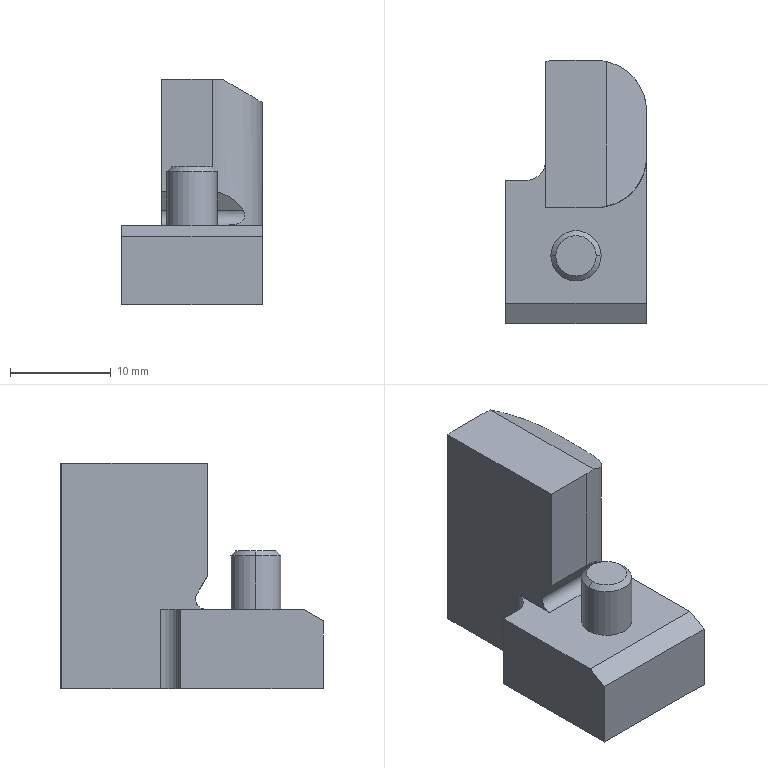Part | SolidWorks | features ICE 6, RefAxis 3, 3DProfileFeature 1, Extrusion 1, RevCut 1, Revolution 1 | 1 solid | 38 faces | box 14 x 26.1 x 22.4 mm | volume 4263 mm3 | plane 23 | cylinder 11 | cone 4 | commonest cylinder face diameters 10 x5 5 x2 8.5 x2 2 x1 4 x1
STEP:
#1=CARTESIAN_POINT('',(2.5,6.7,7.9));
#2=VERTEX_POINT('',#1);
#3=CARTESIAN_POINT('',(-2.5,6.7,7.9));
#4=VERTEX_POINT('',#3);
#5=CARTESIAN_POINT('',(0.,6.7,7.9));
#6=DIRECTION('',(0.,0.,1.));
#7=DIRECTION('',(-1.,0.,0.));
#8=AXIS2_PLACEMENT_3D('',#5,#6,#7);
#9=CIRCLE('',#8,2.5);
#10=EDGE_CURVE('',#2,#4,#9,.T.);
#11=ORIENTED_EDGE('',*,*,#10,.T.);
#12=CARTESIAN_POINT('',(-2.5,6.7,13.21));
#13=VERTEX_POINT('',#12);
#14=CARTESIAN_POINT('',(-2.5,6.7,7.9));
#15=DIRECTION('',(0.,0.,1.));
#16=VECTOR('',#15,1000.);
#17=LINE('',#14,#16);
#18=EDGE_CURVE('',#4,#13,#17,.T.);
#19=ORIENTED_EDGE('',*,*,#18,.T.);
#20=CARTESIAN_POINT('',(2.5,6.7,13.21));
#21=VERTEX_POINT('',#20);
#22=CARTESIAN_POINT('',(0.,6.7,13.21));
#23=DIRECTION('',(0.,0.,1.));
#24=DIRECTION('',(1.,0.,0.));
#25=AXIS2_PLACEMENT_3D('',#22,#23,#24);
#26=CIRCLE('',#25,2.5);
#27=EDGE_CURVE('',#21,#13,#26,.T.);
#28=ORIENTED_EDGE('',*,*,#27,.F.);
#29=CARTESIAN_POINT('',(2.5,6.7,7.9));
#30=DIRECTION('',(0.,0.,1.));
#31=VECTOR('',#30,1000.);
#32=LINE('',#29,#31);
#33=EDGE_CURVE('',#2,#21,#32,.T.);
#34=ORIENTED_EDGE('',*,*,#33,.F.);
#35=EDGE_LOOP('',(#11,#19,#28,#34));
#36=FACE_OUTER_BOUND('',#35,.T.);
#37=CARTESIAN_POINT('',(0.,6.7,7.9));
#38=DIRECTION('',(0.,0.,1.));
#39=DIRECTION('',(1.,0.,0.));
#40=AXIS2_PLACEMENT_3D('',#37,#38,#39);
#41=CYLINDRICAL_SURFACE('',#40,2.5);
#42=ADVANCED_FACE('',(#36),#41,.T.);
#43=CARTESIAN_POINT('',(2.01,6.7,13.7));
#44=VERTEX_POINT('',#43);
#45=CARTESIAN_POINT('',(-2.01,6.7,13.7));
#46=VERTEX_POINT('',#45);
#47=CARTESIAN_POINT('',(0.,6.7,13.7));
#48=DIRECTION('',(0.,0.,1.));
#49=DIRECTION('',(1.,0.,0.));
#50=AXIS2_PLACEMENT_3D('',#47,#48,#49);
#51=CIRCLE('',#50,2.01);
#52=EDGE_CURVE('',#44,#46,#51,.T.);
#53=ORIENTED_EDGE('',*,*,#52,.F.);
#54=CARTESIAN_POINT('',(2.5,6.7,13.21));
#55=DIRECTION('',(0.7071,0.,-0.7071));
#56=VECTOR('',#55,1000.);
#57=LINE('',#54,#56);
#58=EDGE_CURVE('',#44,#21,#57,.T.);
#59=ORIENTED_EDGE('',*,*,#58,.T.);
#60=ORIENTED_EDGE('',*,*,#27,.T.);
#61=CARTESIAN_POINT('',(-2.5,6.7,13.21));
#62=DIRECTION('',(-0.7071,0.,-0.7071));
#63=VECTOR('',#62,1000.);
#64=LINE('',#61,#63);
#65=EDGE_CURVE('',#46,#13,#64,.T.);
#66=ORIENTED_EDGE('',*,*,#65,.F.);
#67=EDGE_LOOP('',(#53,#59,#60,#66));
#68=FACE_OUTER_BOUND('',#67,.T.);
#69=CARTESIAN_POINT('',(0.,6.7,13.21));
#70=DIRECTION('',(0.,0.,-1.));
#71=DIRECTION('',(-1.,0.,0.));
#72=AXIS2_PLACEMENT_3D('',#69,#70,#71);
#73=CONICAL_SURFACE('',#72,2.5,0.7854);
#74=ADVANCED_FACE('',(#68),#73,.T.);
#75=CARTESIAN_POINT('',(-5.,6.7,0.));
#76=VERTEX_POINT('',#75);
#77=CARTESIAN_POINT('',(5.,6.7,0.));
#78=VERTEX_POINT('',#77);
#79=CARTESIAN_POINT('',(0.,6.7,0.));
#80=DIRECTION('',(0.,0.,1.));
#81=DIRECTION('',(1.,0.,0.));
#82=AXIS2_PLACEMENT_3D('',#79,#80,#81);
#83=CIRCLE('',#82,5.);
#84=EDGE_CURVE('',#76,#78,#83,.T.);
#85=ORIENTED_EDGE('',*,*,#84,.F.);
#86=CARTESIAN_POINT('',(-5.,6.7,5.7));
#87=VERTEX_POINT('',#86);
#88=CARTESIAN_POINT('',(-5.,6.7,0.));
#89=DIRECTION('',(0.,0.,1.));
#90=VECTOR('',#89,1000.);
#91=LINE('',#88,#90);
#92=EDGE_CURVE('',#76,#87,#91,.T.);
#93=ORIENTED_EDGE('',*,*,#92,.T.);
#94=CARTESIAN_POINT('',(5.,6.7,5.7));
#95=VERTEX_POINT('',#94);
#96=CARTESIAN_POINT('',(0.,6.7,5.7));
#97=DIRECTION('',(0.,0.,1.));
#98=DIRECTION('',(1.,0.,0.));
#99=AXIS2_PLACEMENT_3D('',#96,#97,#98);
#100=CIRCLE('',#99,5.);
#101=EDGE_CURVE('',#87,#95,#100,.T.);
#102=ORIENTED_EDGE('',*,*,#101,.T.);
#103=CARTESIAN_POINT('',(5.,6.7,0.));
#104=DIRECTION('',(0.,0.,1.));
#105=VECTOR('',#104,1000.);
#106=LINE('',#103,#105);
#107=EDGE_CURVE('',#78,#95,#106,.T.);
#108=ORIENTED_EDGE('',*,*,#107,.F.);
#109=EDGE_LOOP('',(#85,#93,#102,#108));
#110=FACE_OUTER_BOUND('',#109,.T.);
#111=CARTESIAN_POINT('',(0.,6.7,0.));
#112=DIRECTION('',(0.,0.,1.));
#113=DIRECTION('',(1.,0.,0.));
#114=AXIS2_PLACEMENT_3D('',#111,#112,#113);
#115=CYLINDRICAL_SURFACE('',#114,5.);
#116=ADVANCED_FACE('',(#110),#115,.F.);
#117=CARTESIAN_POINT('',(4.25,6.7,1.2));
#118=VERTEX_POINT('',#117);
#119=CARTESIAN_POINT('',(-4.25,6.7,1.2));
#120=VERTEX_POINT('',#119);
#121=CARTESIAN_POINT('',(0.,6.7,1.2));
#122=DIRECTION('',(0.,0.,1.));
#123=DIRECTION('',(1.,0.,0.));
#124=AXIS2_PLACEMENT_3D('',#121,#122,#123);
#125=CIRCLE('',#124,4.25);
#126=EDGE_CURVE('',#118,#120,#125,.T.);
#127=ORIENTED_EDGE('',*,*,#126,.T.);
#128=CARTESIAN_POINT('',(-4.25,6.7,5.7));
#129=VERTEX_POINT('',#128);
#130=CARTESIAN_POINT('',(-4.25,6.7,0.));
#131=DIRECTION('',(0.,0.,1.));
#132=VECTOR('',#131,1000.);
#133=LINE('',#130,#132);
#134=EDGE_CURVE('',#120,#129,#133,.T.);
#135=ORIENTED_EDGE('',*,*,#134,.T.);
#136=CARTESIAN_POINT('',(4.25,6.7,5.7));
#137=VERTEX_POINT('',#136);
#138=CARTESIAN_POINT('',(0.,6.7,5.7));
#139=DIRECTION('',(0.,0.,1.));
#140=DIRECTION('',(1.,0.,0.));
#141=AXIS2_PLACEMENT_3D('',#138,#139,#140);
#142=CIRCLE('',#141,4.25);
#143=EDGE_CURVE('',#137,#129,#142,.T.);
#144=ORIENTED_EDGE('',*,*,#143,.F.);
#145=CARTESIAN_POINT('',(4.25,6.7,0.));
#146=DIRECTION('',(0.,0.,1.));
#147=VECTOR('',#146,1000.);
#148=LINE('',#145,#147);
#149=EDGE_CURVE('',#118,#137,#148,.T.);
#150=ORIENTED_EDGE('',*,*,#149,.F.);
#151=EDGE_LOOP('',(#127,#135,#144,#150));
#152=FACE_OUTER_BOUND('',#151,.T.);
#153=CARTESIAN_POINT('',(0.,6.7,0.));
#154=DIRECTION('',(0.,0.,1.));
#155=DIRECTION('',(1.,0.,0.));
#156=AXIS2_PLACEMENT_3D('',#153,#154,#155);
#157=CYLINDRICAL_SURFACE('',#156,4.25);
#158=ADVANCED_FACE('',(#152),#157,.T.);
#159=CARTESIAN_POINT('',(3.75,6.7,0.7));
#160=VERTEX_POINT('',#159);
#161=CARTESIAN_POINT('',(-3.75,6.7,0.7));
#162=VERTEX_POINT('',#161);
#163=CARTESIAN_POINT('',(0.,6.7,0.7));
#164=DIRECTION('',(0.,0.,1.));
#165=DIRECTION('',(1.,0.,0.));
#166=AXIS2_PLACEMENT_3D('',#163,#164,#165);
#167=CIRCLE('',#166,3.75);
#168=EDGE_CURVE('',#160,#162,#167,.T.);
#169=ORIENTED_EDGE('',*,*,#168,.T.);
#170=CARTESIAN_POINT('',(-4.25,6.7,1.2));
#171=DIRECTION('',(-0.7071,0.,0.7071));
#172=VECTOR('',#171,1000.);
#173=LINE('',#170,#172);
#174=EDGE_CURVE('',#162,#120,#173,.T.);
#175=ORIENTED_EDGE('',*,*,#174,.T.);
#176=ORIENTED_EDGE('',*,*,#126,.F.);
#177=CARTESIAN_POINT('',(4.25,6.7,1.2));
#178=DIRECTION('',(0.7071,0.,0.7071));
#179=VECTOR('',#178,1000.);
#180=LINE('',#177,#179);
#181=EDGE_CURVE('',#160,#118,#180,.T.);
#182=ORIENTED_EDGE('',*,*,#181,.F.);
#183=EDGE_LOOP('',(#169,#175,#176,#182));
#184=FACE_OUTER_BOUND('',#183,.T.);
#185=CARTESIAN_POINT('',(0.,6.7,1.2));
#186=DIRECTION('',(0.,0.,1.));
#187=DIRECTION('',(1.,0.,0.));
#188=AXIS2_PLACEMENT_3D('',#185,#186,#187);
#189=CONICAL_SURFACE('',#188,4.25,0.7854);
#190=ADVANCED_FACE('',(#184),#189,.T.);
#191=CARTESIAN_POINT('',(-3.,11.7,7.9));
#192=VERTEX_POINT('',#191);
#193=CARTESIAN_POINT('',(3.4,11.7,7.9));
#194=VERTEX_POINT('',#193);
#195=CARTESIAN_POINT('',(-7.,11.7,7.9));
#196=DIRECTION('',(1.,0.,0.));
#197=VECTOR('',#196,1000.);
#198=LINE('',#195,#197);
#199=EDGE_CURVE('',#192,#194,#198,.T.);
#200=ORIENTED_EDGE('',*,*,#199,.F.);
#201=CARTESIAN_POINT('',(-3.,16.2,7.9));
#202=VERTEX_POINT('',#201);
#203=CARTESIAN_POINT('',(-3.,11.5,7.9));
#204=DIRECTION('',(0.,1.,0.));
#205=VECTOR('',#204,1000.);
#206=LINE('',#203,#205);
#207=EDGE_CURVE('',#192,#202,#206,.T.);
#208=ORIENTED_EDGE('',*,*,#207,.T.);
#209=CARTESIAN_POINT('',(-5.,14.2,7.9));
#210=VERTEX_POINT('',#209);
#211=CARTESIAN_POINT('',(-5.,16.2,7.9));
#212=DIRECTION('',(0.,0.,-1.));
#213=DIRECTION('',(-1.,0.,0.));
#214=AXIS2_PLACEMENT_3D('',#211,#212,#213);
#215=CIRCLE('',#214,2.);
#216=EDGE_CURVE('',#202,#210,#215,.T.);
#217=ORIENTED_EDGE('',*,*,#216,.T.);
#218=CARTESIAN_POINT('',(-7.,14.2,7.9));
#219=VERTEX_POINT('',#218);
#220=CARTESIAN_POINT('',(2.,14.2,7.9));
#221=DIRECTION('',(-1.,0.,0.));
#222=VECTOR('',#221,1000.);
#223=LINE('',#220,#222);
#224=EDGE_CURVE('',#210,#219,#223,.T.);
#225=ORIENTED_EDGE('',*,*,#224,.T.);
#226=CARTESIAN_POINT('',(-7.,2.,7.9));
#227=VERTEX_POINT('',#226);
#228=CARTESIAN_POINT('',(-7.,26.1,7.9));
#229=DIRECTION('',(0.,-1.,0.));
#230=VECTOR('',#229,1000.);
#231=LINE('',#228,#230);
#232=EDGE_CURVE('',#219,#227,#231,.T.);
#233=ORIENTED_EDGE('',*,*,#232,.T.);
#234=CARTESIAN_POINT('',(7.,2.,7.9));
#235=VERTEX_POINT('',#234);
#236=CARTESIAN_POINT('',(-7.,2.,7.9));
#237=DIRECTION('',(1.,0.,0.));
#238=VECTOR('',#237,1000.);
#239=LINE('',#236,#238);
#240=EDGE_CURVE('',#227,#235,#239,.T.);
#241=ORIENTED_EDGE('',*,*,#240,.T.);
#242=CARTESIAN_POINT('',(7.,16.5,7.9));
#243=VERTEX_POINT('',#242);
#244=CARTESIAN_POINT('',(7.,0.,7.9));
#245=DIRECTION('',(0.,-1.,0.));
#246=VECTOR('',#245,1000.);
#247=LINE('',#244,#246);
#248=EDGE_CURVE('',#243,#235,#247,.T.);
#249=ORIENTED_EDGE('',*,*,#248,.F.);
#250=CARTESIAN_POINT('',(2.,16.5,7.9));
#251=DIRECTION('',(0.,0.,-1.));
#252=DIRECTION('',(-1.,0.,0.));
#253=AXIS2_PLACEMENT_3D('',#250,#251,#252);
#254=CIRCLE('',#253,5.);
#255=EDGE_CURVE('',#243,#194,#254,.T.);
#256=ORIENTED_EDGE('',*,*,#255,.T.);
#257=EDGE_LOOP('',(#200,#208,#217,#225,#233,#241,#249,#256));
#258=FACE_OUTER_BOUND('',#257,.T.);
#259=ORIENTED_EDGE('',*,*,#10,.F.);
#260=CARTESIAN_POINT('',(0.,6.7,7.9));
#261=DIRECTION('',(0.,0.,1.));
#262=DIRECTION('',(-1.,0.,0.));
#263=AXIS2_PLACEMENT_3D('',#260,#261,#262);
#264=CIRCLE('',#263,2.5);
#265=EDGE_CURVE('',#4,#2,#264,.T.);
#266=ORIENTED_EDGE('',*,*,#265,.F.);
#267=EDGE_LOOP('',(#259,#266));
#268=FACE_BOUND('',#267,.T.);
#269=CARTESIAN_POINT('',(2.,16.5,7.9));
#270=DIRECTION('',(0.,0.,-1.));
#271=DIRECTION('',(-1.,0.,0.));
#272=AXIS2_PLACEMENT_3D('',#269,#270,#271);
#273=PLANE('',#272);
#274=ADVANCED_FACE('',(#258,#268),#273,.F.);
#275=CARTESIAN_POINT('',(-5.,14.2,0.));
#276=VERTEX_POINT('',#275);
#277=CARTESIAN_POINT('',(-3.,16.2,0.));
#278=VERTEX_POINT('',#277);
#279=CARTESIAN_POINT('',(-5.,16.2,0.));
#280=DIRECTION('',(0.,0.,1.));
#281=DIRECTION('',(1.,0.,0.));
#282=AXIS2_PLACEMENT_3D('',#279,#280,#281);
#283=CIRCLE('',#282,2.);
#284=EDGE_CURVE('',#276,#278,#283,.T.);
#285=ORIENTED_EDGE('',*,*,#284,.T.);
#286=CARTESIAN_POINT('',(-3.,25.999,0.));
#287=VERTEX_POINT('',#286);
#288=CARTESIAN_POINT('',(-3.,16.2,0.));
#289=DIRECTION('',(0.,1.,0.));
#290=VECTOR('',#289,1000.);
#291=LINE('',#288,#290);
#292=EDGE_CURVE('',#278,#287,#291,.T.);
#293=ORIENTED_EDGE('',*,*,#292,.T.);
#294=CARTESIAN_POINT('',(-2.,26.1,0.));
#295=VERTEX_POINT('',#294);
#296=CARTESIAN_POINT('',(-2.,21.1,0.));
#297=DIRECTION('',(0.,0.,1.));
#298=DIRECTION('',(1.,0.,0.));
#299=AXIS2_PLACEMENT_3D('',#296,#297,#298);
#300=CIRCLE('',#299,5.);
#301=EDGE_CURVE('',#295,#287,#300,.T.);
#302=ORIENTED_EDGE('',*,*,#301,.F.);
#303=CARTESIAN_POINT('',(2.,26.1,0.));
#304=VERTEX_POINT('',#303);
#305=CARTESIAN_POINT('',(2.,26.1,0.));
#306=DIRECTION('',(-1.,0.,0.));
#307=VECTOR('',#306,1000.);
#308=LINE('',#305,#307);
#309=EDGE_CURVE('',#304,#295,#308,.T.);
#310=ORIENTED_EDGE('',*,*,#309,.F.);
#311=CARTESIAN_POINT('',(7.,21.1,0.));
#312=VERTEX_POINT('',#311);
#313=CARTESIAN_POINT('',(2.,21.1,0.));
#314=DIRECTION('',(0.,0.,1.));
#315=DIRECTION('',(1.,0.,0.));
#316=AXIS2_PLACEMENT_3D('',#313,#314,#315);
#317=CIRCLE('',#316,5.);
#318=EDGE_CURVE('',#312,#304,#317,.T.);
#319=ORIENTED_EDGE('',*,*,#318,.F.);
#320=CARTESIAN_POINT('',(7.,0.,0.));
#321=VERTEX_POINT('',#320);
#322=CARTESIAN_POINT('',(7.,0.,0.));
#323=DIRECTION('',(0.,1.,0.));
#324=VECTOR('',#323,1000.);
#325=LINE('',#322,#324);
#326=EDGE_CURVE('',#321,#312,#325,.T.);
#327=ORIENTED_EDGE('',*,*,#326,.F.);
#328=CARTESIAN_POINT('',(-7.,0.,0.));
#329=VERTEX_POINT('',#328);
#330=CARTESIAN_POINT('',(-7.,0.,0.));
#331=DIRECTION('',(1.,0.,0.));
#332=VECTOR('',#331,1000.);
#333=LINE('',#330,#332);
#334=EDGE_CURVE('',#329,#321,#333,.T.);
#335=ORIENTED_EDGE('',*,*,#334,.F.);
#336=CARTESIAN_POINT('',(-7.,14.2,0.));
#337=VERTEX_POINT('',#336);
#338=CARTESIAN_POINT('',(-7.,21.1,0.));
#339=DIRECTION('',(0.,-1.,0.));
#340=VECTOR('',#339,1000.);
#341=LINE('',#338,#340);
#342=EDGE_CURVE('',#337,#329,#341,.T.);
#343=ORIENTED_EDGE('',*,*,#342,.F.);
#344=CARTESIAN_POINT('',(-7.,14.2,0.));
#345=DIRECTION('',(1.,0.,0.));
#346=VECTOR('',#345,1000.);
#347=LINE('',#344,#346);
#348=EDGE_CURVE('',#337,#276,#347,.T.);
#349=ORIENTED_EDGE('',*,*,#348,.T.);
#350=EDGE_LOOP('',(#285,#293,#302,#310,#319,#327,#335,#343,#349));
#351=FACE_OUTER_BOUND('',#350,.T.);
#352=CARTESIAN_POINT('',(0.,6.7,0.));
#353=DIRECTION('',(0.,0.,1.));
#354=DIRECTION('',(1.,0.,0.));
#355=AXIS2_PLACEMENT_3D('',#352,#353,#354);
#356=CIRCLE('',#355,5.);
#357=EDGE_CURVE('',#78,#76,#356,.T.);
#358=ORIENTED_EDGE('',*,*,#357,.T.);
#359=ORIENTED_EDGE('',*,*,#84,.T.);
#360=EDGE_LOOP('',(#358,#359));
#361=FACE_BOUND('',#360,.T.);
#362=CARTESIAN_POINT('',(-2.,21.1,0.));
#363=DIRECTION('',(0.,0.,1.));
#364=DIRECTION('',(1.,0.,0.));
#365=AXIS2_PLACEMENT_3D('',#362,#363,#364);
#366=PLANE('',#365);
#367=ADVANCED_FACE('',(#351,#361),#366,.F.);
#368=ORIENTED_EDGE('',*,*,#301,.T.);
#369=CARTESIAN_POINT('',(-3.,25.999,22.4));
#370=VERTEX_POINT('',#369);
#371=CARTESIAN_POINT('',(-3.,25.999,22.4));
#372=DIRECTION('',(0.,0.,-1.));
#373=VECTOR('',#372,1000.);
#374=LINE('',#371,#373);
#375=EDGE_CURVE('',#370,#287,#374,.T.);
#376=ORIENTED_EDGE('',*,*,#375,.F.);
#377=CARTESIAN_POINT('',(-2.,26.1,22.4));
#378=VERTEX_POINT('',#377);
#379=CARTESIAN_POINT('',(-2.,21.1,22.4));
#380=DIRECTION('',(0.,0.,1.));
#381=DIRECTION('',(1.,0.,0.));
#382=AXIS2_PLACEMENT_3D('',#379,#380,#381);
#383=CIRCLE('',#382,5.);
#384=EDGE_CURVE('',#378,#370,#383,.T.);
#385=ORIENTED_EDGE('',*,*,#384,.F.);
#386=CARTESIAN_POINT('',(-2.,26.1,22.4));
#387=DIRECTION('',(0.,0.,-1.));
#388=VECTOR('',#387,1000.);
#389=LINE('',#386,#388);
#390=EDGE_CURVE('',#378,#295,#389,.T.);
#391=ORIENTED_EDGE('',*,*,#390,.T.);
#392=EDGE_LOOP('',(#368,#376,#385,#391));
#393=FACE_OUTER_BOUND('',#392,.T.);
#394=CARTESIAN_POINT('',(-2.,21.1,22.4));
#395=DIRECTION('',(0.,0.,-1.));
#396=DIRECTION('',(-1.,0.,0.));
#397=AXIS2_PLACEMENT_3D('',#394,#395,#396);
#398=CYLINDRICAL_SURFACE('',#397,5.);
#399=ADVANCED_FACE('',(#393),#398,.T.);
#400=CARTESIAN_POINT('',(3.016,11.604,22.4));
#401=VERTEX_POINT('',#400);
#402=CARTESIAN_POINT('',(3.016,25.996,22.4));
#403=VERTEX_POINT('',#402);
#404=CARTESIAN_POINT('',(3.016,-26.1,22.4));
#405=DIRECTION('',(0.,1.,0.));
#406=VECTOR('',#405,1000.);
#407=LINE('',#404,#406);
#408=EDGE_CURVE('',#401,#403,#407,.T.);
#409=ORIENTED_EDGE('',*,*,#408,.T.);
#410=CARTESIAN_POINT('',(2.,26.1,22.4));
#411=VERTEX_POINT('',#410);
#412=CARTESIAN_POINT('',(2.,21.1,22.4));
#413=DIRECTION('',(0.,0.,1.));
#414=DIRECTION('',(1.,0.,0.));
#415=AXIS2_PLACEMENT_3D('',#412,#413,#414);
#416=CIRCLE('',#415,5.);
#417=EDGE_CURVE('',#403,#411,#416,.T.);
#418=ORIENTED_EDGE('',*,*,#417,.T.);
#419=CARTESIAN_POINT('',(2.,26.1,22.4));
#420=DIRECTION('',(-1.,0.,0.));
#421=VECTOR('',#420,1000.);
#422=LINE('',#419,#421);
#423=EDGE_CURVE('',#411,#378,#422,.T.);
#424=ORIENTED_EDGE('',*,*,#423,.T.);
#425=ORIENTED_EDGE('',*,*,#384,.T.);
#426=CARTESIAN_POINT('',(-3.,11.5,22.4));
#427=VERTEX_POINT('',#426);
#428=CARTESIAN_POINT('',(-3.,21.1,22.4));
#429=DIRECTION('',(0.,-1.,0.));
#430=VECTOR('',#429,1000.);
#431=LINE('',#428,#430);
#432=EDGE_CURVE('',#370,#427,#431,.T.);
#433=ORIENTED_EDGE('',*,*,#432,.T.);
#434=CARTESIAN_POINT('',(2.,11.5,22.4));
#435=VERTEX_POINT('',#434);
#436=CARTESIAN_POINT('',(-2.,11.5,22.4));
#437=DIRECTION('',(1.,0.,0.));
#438=VECTOR('',#437,1000.);
#439=LINE('',#436,#438);
#440=EDGE_CURVE('',#427,#435,#439,.T.);
#441=ORIENTED_EDGE('',*,*,#440,.T.);
#442=CARTESIAN_POINT('',(2.,16.5,22.4));
#443=DIRECTION('',(0.,0.,1.));
#444=DIRECTION('',(1.,0.,0.));
#445=AXIS2_PLACEMENT_3D('',#442,#443,#444);
#446=CIRCLE('',#445,5.);
#447=EDGE_CURVE('',#435,#401,#446,.T.);
#448=ORIENTED_EDGE('',*,*,#447,.T.);
#449=EDGE_LOOP('',(#409,#418,#424,#425,#433,#441,#448));
#450=FACE_OUTER_BOUND('',#449,.T.);
#451=CARTESIAN_POINT('',(-2.,21.1,22.4));
#452=DIRECTION('',(0.,0.,1.));
#453=DIRECTION('',(1.,0.,0.));
#454=AXIS2_PLACEMENT_3D('',#451,#452,#453);
#455=PLANE('',#454);
#456=ADVANCED_FACE('',(#450),#455,.T.);
#457=CARTESIAN_POINT('',(7.,0.,6.745));
#458=VERTEX_POINT('',#457);
#459=CARTESIAN_POINT('',(7.,0.,22.4));
#460=DIRECTION('',(0.,0.,-1.));
#461=VECTOR('',#460,1000.);
#462=LINE('',#459,#461);
#463=EDGE_CURVE('',#458,#321,#462,.T.);
#464=ORIENTED_EDGE('',*,*,#463,.F.);
#465=CARTESIAN_POINT('',(-7.,0.,6.745));
#466=VERTEX_POINT('',#465);
#467=CARTESIAN_POINT('',(-7.,0.,6.745));
#468=DIRECTION('',(1.,0.,0.));
#469=VECTOR('',#468,1000.);
#470=LINE('',#467,#469);
#471=EDGE_CURVE('',#466,#458,#470,.T.);
#472=ORIENTED_EDGE('',*,*,#471,.F.);
#473=CARTESIAN_POINT('',(-7.,0.,22.4));
#474=DIRECTION('',(0.,0.,-1.));
#475=VECTOR('',#474,1000.);
#476=LINE('',#473,#475);
#477=EDGE_CURVE('',#466,#329,#476,.T.);
#478=ORIENTED_EDGE('',*,*,#477,.T.);
#479=ORIENTED_EDGE('',*,*,#334,.T.);
#480=EDGE_LOOP('',(#464,#472,#478,#479));
#481=FACE_OUTER_BOUND('',#480,.T.);
#482=CARTESIAN_POINT('',(-7.,0.,22.4));
#483=DIRECTION('',(0.,1.,0.));
#484=DIRECTION('',(0.,0.,1.));
#485=AXIS2_PLACEMENT_3D('',#482,#483,#484);
#486=PLANE('',#485);
#487=ADVANCED_FACE('',(#481),#486,.F.);
#488=ORIENTED_EDGE('',*,*,#232,.F.);
#489=CARTESIAN_POINT('',(-7.,14.2,0.));
#490=DIRECTION('',(0.,0.,1.));
#491=VECTOR('',#490,1000.);
#492=LINE('',#489,#491);
#493=EDGE_CURVE('',#337,#219,#492,.T.);
#494=ORIENTED_EDGE('',*,*,#493,.F.);
#495=ORIENTED_EDGE('',*,*,#342,.T.);
#496=ORIENTED_EDGE('',*,*,#477,.F.);
#497=CARTESIAN_POINT('',(-7.,0.,6.745));
#498=DIRECTION('',(0.,0.866,0.5));
#499=VECTOR('',#498,1000.);
#500=LINE('',#497,#499);
#501=EDGE_CURVE('',#466,#227,#500,.T.);
#502=ORIENTED_EDGE('',*,*,#501,.T.);
#503=EDGE_LOOP('',(#488,#494,#495,#496,#502));
#504=FACE_OUTER_BOUND('',#503,.T.);
#505=CARTESIAN_POINT('',(-7.,21.1,22.4));
#506=DIRECTION('',(1.,0.,0.));
#507=DIRECTION('',(0.,0.,-1.));
#508=AXIS2_PLACEMENT_3D('',#505,#506,#507);
#509=PLANE('',#508);
#510=ADVANCED_FACE('',(#504),#509,.F.);
#511=CARTESIAN_POINT('',(7.,21.1,20.1));
#512=VERTEX_POINT('',#511);
#513=CARTESIAN_POINT('',(7.,21.1,22.4));
#514=DIRECTION('',(0.,0.,-1.));
#515=VECTOR('',#514,1000.);
#516=LINE('',#513,#515);
#517=EDGE_CURVE('',#512,#312,#516,.T.);
#518=ORIENTED_EDGE('',*,*,#517,.F.);
#519=CARTESIAN_POINT('',(7.,16.5,20.1));
#520=VERTEX_POINT('',#519);
#521=CARTESIAN_POINT('',(7.,-26.1,20.1));
#522=DIRECTION('',(0.,1.,0.));
#523=VECTOR('',#522,1000.);
#524=LINE('',#521,#523);
#525=EDGE_CURVE('',#520,#512,#524,.T.);
#526=ORIENTED_EDGE('',*,*,#525,.F.);
#527=CARTESIAN_POINT('',(7.,16.5,27.7));
#528=DIRECTION('',(0.,0.,-1.));
#529=VECTOR('',#528,1000.);
#530=LINE('',#527,#529);
#531=EDGE_CURVE('',#520,#243,#530,.T.);
#532=ORIENTED_EDGE('',*,*,#531,.T.);
#533=ORIENTED_EDGE('',*,*,#248,.T.);
#534=CARTESIAN_POINT('',(7.,0.,6.745));
#535=DIRECTION('',(0.,0.866,0.5));
#536=VECTOR('',#535,1000.);
#537=LINE('',#534,#536);
#538=EDGE_CURVE('',#458,#235,#537,.T.);
#539=ORIENTED_EDGE('',*,*,#538,.F.);
#540=ORIENTED_EDGE('',*,*,#463,.T.);
#541=ORIENTED_EDGE('',*,*,#326,.T.);
#542=EDGE_LOOP('',(#518,#526,#532,#533,#539,#540,#541));
#543=FACE_OUTER_BOUND('',#542,.T.);
#544=CARTESIAN_POINT('',(7.,0.,22.4));
#545=DIRECTION('',(-1.,0.,0.));
#546=DIRECTION('',(0.,0.,1.));
#547=AXIS2_PLACEMENT_3D('',#544,#545,#546);
#548=PLANE('',#547);
#549=ADVANCED_FACE('',(#543),#548,.F.);
#550=ORIENTED_EDGE('',*,*,#417,.F.);
#551=CARTESIAN_POINT('',(3.016,25.996,22.4));
#552=CARTESIAN_POINT('',(5.439,25.493,21.002));
#553=CARTESIAN_POINT('',(7.,23.574,20.1));
#554=CARTESIAN_POINT('',(7.,21.1,20.1));
#555=(BOUNDED_CURVE()B_SPLINE_CURVE(3,(#551,#552,#553,#554),.UNSPECIFIED.,.F.,.F.)B_SPLINE_CURVE_WITH_KNOTS((4,4),(4.917,6.283),.UNSPECIFIED.)CURVE()GEOMETRIC_REPRESENTATION_ITEM()RATIONAL_B_SPLINE_CURVE((1.,0.8504,0.8504,1.))REPRESENTATION_ITEM(''));
#556=EDGE_CURVE('',#403,#512,#555,.T.);
#557=ORIENTED_EDGE('',*,*,#556,.T.);
#558=ORIENTED_EDGE('',*,*,#517,.T.);
#559=ORIENTED_EDGE('',*,*,#318,.T.);
#560=CARTESIAN_POINT('',(2.,26.1,22.4));
#561=DIRECTION('',(0.,0.,-1.));
#562=VECTOR('',#561,1000.);
#563=LINE('',#560,#562);
#564=EDGE_CURVE('',#411,#304,#563,.T.);
#565=ORIENTED_EDGE('',*,*,#564,.F.);
#566=EDGE_LOOP('',(#550,#557,#558,#559,#565));
#567=FACE_OUTER_BOUND('',#566,.T.);
#568=CARTESIAN_POINT('',(2.,21.1,22.4));
#569=DIRECTION('',(0.,0.,-1.));
#570=DIRECTION('',(-1.,0.,0.));
#571=AXIS2_PLACEMENT_3D('',#568,#569,#570);
#572=CYLINDRICAL_SURFACE('',#571,5.);
#573=ADVANCED_FACE('',(#567),#572,.T.);
#574=ORIENTED_EDGE('',*,*,#309,.T.);
#575=ORIENTED_EDGE('',*,*,#390,.F.);
#576=ORIENTED_EDGE('',*,*,#423,.F.);
#577=ORIENTED_EDGE('',*,*,#564,.T.);
#578=EDGE_LOOP('',(#574,#575,#576,#577));
#579=FACE_OUTER_BOUND('',#578,.T.);
#580=CARTESIAN_POINT('',(2.,26.1,22.4));
#581=DIRECTION('',(0.,-1.,0.));
#582=DIRECTION('',(0.,0.,-1.));
#583=AXIS2_PLACEMENT_3D('',#580,#581,#582);
#584=PLANE('',#583);
#585=ADVANCED_FACE('',(#579),#584,.F.);
#586=ORIENTED_EDGE('',*,*,#240,.F.);
#587=ORIENTED_EDGE('',*,*,#501,.F.);
#588=ORIENTED_EDGE('',*,*,#471,.T.);
#589=ORIENTED_EDGE('',*,*,#538,.T.);
#590=EDGE_LOOP('',(#586,#587,#588,#589));
#591=FACE_OUTER_BOUND('',#590,.T.);
#592=CARTESIAN_POINT('',(-7.,0.,6.745));
#593=DIRECTION('',(0.,0.5,-0.866));
#594=DIRECTION('',(0.,0.866,0.5));
#595=AXIS2_PLACEMENT_3D('',#592,#593,#594);
#596=PLANE('',#595);
#597=ADVANCED_FACE('',(#591),#596,.F.);
#598=CARTESIAN_POINT('',(-3.,11.5,11.246));
#599=VERTEX_POINT('',#598);
#600=CARTESIAN_POINT('',(-3.,12.566,9.4));
#601=VERTEX_POINT('',#600);
#602=CARTESIAN_POINT('',(-3.,4.375,23.587));
#603=DIRECTION('',(0.,0.5,-0.866));
#604=VECTOR('',#603,1000.);
#605=LINE('',#602,#604);
#606=EDGE_CURVE('',#599,#601,#605,.T.);
#607=ORIENTED_EDGE('',*,*,#606,.F.);
#608=CARTESIAN_POINT('',(-3.,11.5,27.7));
#609=DIRECTION('',(0.,0.,-1.));
#610=VECTOR('',#609,1000.);
#611=LINE('',#608,#610);
#612=EDGE_CURVE('',#427,#599,#611,.T.);
#613=ORIENTED_EDGE('',*,*,#612,.F.);
#614=ORIENTED_EDGE('',*,*,#432,.F.);
#615=ORIENTED_EDGE('',*,*,#375,.T.);
#616=ORIENTED_EDGE('',*,*,#292,.F.);
#617=CARTESIAN_POINT('',(-3.,16.2,0.));
#618=DIRECTION('',(0.,0.,1.));
#619=VECTOR('',#618,1000.);
#620=LINE('',#617,#619);
#621=EDGE_CURVE('',#278,#202,#620,.T.);
#622=ORIENTED_EDGE('',*,*,#621,.T.);
#623=ORIENTED_EDGE('',*,*,#207,.F.);
#624=CARTESIAN_POINT('',(-3.,11.7,8.9));
#625=DIRECTION('',(-1.,0.,0.));
#626=DIRECTION('',(0.,-1.,0.));
#627=AXIS2_PLACEMENT_3D('',#624,#625,#626);
#628=CIRCLE('',#627,1.);
#629=EDGE_CURVE('',#601,#192,#628,.T.);
#630=ORIENTED_EDGE('',*,*,#629,.F.);
#631=EDGE_LOOP('',(#607,#613,#614,#615,#616,#622,#623,#630));
#632=FACE_OUTER_BOUND('',#631,.T.);
#633=CARTESIAN_POINT('',(-3.,11.5,27.7));
#634=DIRECTION('',(-1.,0.,0.));
#635=DIRECTION('',(0.,-1.,0.));
#636=AXIS2_PLACEMENT_3D('',#633,#634,#635);
#637=PLANE('',#636);
#638=ADVANCED_FACE('',(#632),#637,.T.);
#639=CARTESIAN_POINT('',(3.016,11.604,22.4));
#640=CARTESIAN_POINT('',(5.439,12.107,21.002));
#641=CARTESIAN_POINT('',(7.,14.026,20.1));
#642=CARTESIAN_POINT('',(7.,16.5,20.1));
#643=(BOUNDED_CURVE()B_SPLINE_CURVE(3,(#639,#640,#641,#642),.UNSPECIFIED.,.F.,.T.)B_SPLINE_CURVE_WITH_KNOTS((4,4),(4.917,6.283),.UNSPECIFIED.)CURVE()GEOMETRIC_REPRESENTATION_ITEM()RATIONAL_B_SPLINE_CURVE((1.,0.8504,0.8504,1.))REPRESENTATION_ITEM(''));
#644=EDGE_CURVE('',#401,#520,#643,.T.);
#645=ORIENTED_EDGE('',*,*,#644,.F.);
#646=ORIENTED_EDGE('',*,*,#447,.F.);
#647=CARTESIAN_POINT('',(2.,11.5,11.246));
#648=VERTEX_POINT('',#647);
#649=CARTESIAN_POINT('',(2.,11.5,27.7));
#650=DIRECTION('',(0.,0.,-1.));
#651=VECTOR('',#650,1000.);
#652=LINE('',#649,#651);
#653=EDGE_CURVE('',#435,#648,#652,.T.);
#654=ORIENTED_EDGE('',*,*,#653,.T.);
#655=CARTESIAN_POINT('',(5.086,12.566,9.4));
#656=VERTEX_POINT('',#655);
#657=CARTESIAN_POINT('',(5.086,12.566,9.4));
#658=CARTESIAN_POINT('',(4.197,11.869,10.608));
#659=CARTESIAN_POINT('',(3.13,11.5,11.246));
#660=CARTESIAN_POINT('',(2.,11.5,11.246));
#661=(BOUNDED_CURVE()B_SPLINE_CURVE(3,(#657,#658,#659,#660),.UNSPECIFIED.,.F.,.F.)B_SPLINE_CURVE_WITH_KNOTS((4,4),(2.476,3.142),.UNSPECIFIED.)CURVE()GEOMETRIC_REPRESENTATION_ITEM()RATIONAL_B_SPLINE_CURVE((1.,0.9635,0.9635,1.))REPRESENTATION_ITEM(''));
#662=EDGE_CURVE('',#656,#648,#661,.T.);
#663=ORIENTED_EDGE('',*,*,#662,.F.);
#664=CARTESIAN_POINT('',(3.4,11.7,7.9));
#665=CARTESIAN_POINT('',(3.651,11.773,7.9));
#666=CARTESIAN_POINT('',(3.894,11.865,7.907));
#667=CARTESIAN_POINT('',(4.361,12.085,7.97));
#668=CARTESIAN_POINT('',(4.588,12.215,8.026));
#669=CARTESIAN_POINT('',(4.882,12.412,8.193));
#670=CARTESIAN_POINT('',(4.972,12.478,8.263));
#671=CARTESIAN_POINT('',(5.124,12.595,8.442));
#672=CARTESIAN_POINT('',(5.185,12.645,8.551));
#673=CARTESIAN_POINT('',(5.253,12.703,8.797));
#674=CARTESIAN_POINT('',(5.259,12.708,8.934));
#675=CARTESIAN_POINT('',(5.21,12.666,9.188));
#676=CARTESIAN_POINT('',(5.157,12.622,9.304));
#677=CARTESIAN_POINT('',(5.086,12.566,9.4));
#678=B_SPLINE_CURVE_WITH_KNOTS('',3,(#664,#665,#666,#667,#668,#669,#670,#671,#672,#673,#674,#675,#676,#677),.UNSPECIFIED.,.F.,.F.,(4,2,2,2,2,2,4),(0.,0.000778,0.001556,0.001945,0.002334,0.002723,0.003112),.UNSPECIFIED.);
#679=EDGE_CURVE('',#194,#656,#678,.T.);
#680=ORIENTED_EDGE('',*,*,#679,.F.);
#681=ORIENTED_EDGE('',*,*,#255,.F.);
#682=ORIENTED_EDGE('',*,*,#531,.F.);
#683=EDGE_LOOP('',(#645,#646,#654,#663,#680,#681,#682));
#684=FACE_OUTER_BOUND('',#683,.T.);
#685=CARTESIAN_POINT('',(2.,16.5,27.7));
#686=DIRECTION('',(0.,0.,-1.));
#687=DIRECTION('',(-1.,0.,0.));
#688=AXIS2_PLACEMENT_3D('',#685,#686,#687);
#689=CYLINDRICAL_SURFACE('',#688,5.);
#690=ADVANCED_FACE('',(#684),#689,.T.);
#691=CARTESIAN_POINT('',(2.,11.5,11.246));
#692=DIRECTION('',(-1.,0.,0.));
#693=VECTOR('',#692,1000.);
#694=LINE('',#691,#693);
#695=EDGE_CURVE('',#648,#599,#694,.T.);
#696=ORIENTED_EDGE('',*,*,#695,.F.);
#697=ORIENTED_EDGE('',*,*,#653,.F.);
#698=ORIENTED_EDGE('',*,*,#440,.F.);
#699=ORIENTED_EDGE('',*,*,#612,.T.);
#700=EDGE_LOOP('',(#696,#697,#698,#699));
#701=FACE_OUTER_BOUND('',#700,.T.);
#702=CARTESIAN_POINT('',(2.,11.5,27.7));
#703=DIRECTION('',(0.,-1.,0.));
#704=DIRECTION('',(0.,0.,-1.));
#705=AXIS2_PLACEMENT_3D('',#702,#703,#704);
#706=PLANE('',#705);
#707=ADVANCED_FACE('',(#701),#706,.T.);
#708=CARTESIAN_POINT('',(1.155,4.7,0.7));
#709=VERTEX_POINT('',#708);
#710=CARTESIAN_POINT('',(-1.155,4.7,0.7));
#711=VERTEX_POINT('',#710);
#712=CARTESIAN_POINT('',(1.155,4.7,0.7));
#713=DIRECTION('',(-1.,0.,0.));
#714=VECTOR('',#713,1000.);
#715=LINE('',#712,#714);
#716=EDGE_CURVE('',#709,#711,#715,.T.);
#717=ORIENTED_EDGE('',*,*,#716,.F.);
#718=CARTESIAN_POINT('',(2.309,6.7,0.7));
#719=VERTEX_POINT('',#718);
#720=CARTESIAN_POINT('',(2.309,6.7,0.7));
#721=DIRECTION('',(-0.5,-0.866,0.));
#722=VECTOR('',#721,1000.);
#723=LINE('',#720,#722);
#724=EDGE_CURVE('',#719,#709,#723,.T.);
#725=ORIENTED_EDGE('',*,*,#724,.F.);
#726=CARTESIAN_POINT('',(1.155,8.7,0.7));
#727=VERTEX_POINT('',#726);
#728=CARTESIAN_POINT('',(1.155,8.7,0.7));
#729=DIRECTION('',(0.5,-0.866,0.));
#730=VECTOR('',#729,1000.);
#731=LINE('',#728,#730);
#732=EDGE_CURVE('',#727,#719,#731,.T.);
#733=ORIENTED_EDGE('',*,*,#732,.F.);
#734=CARTESIAN_POINT('',(-1.155,8.7,0.7));
#735=VERTEX_POINT('',#734);
#736=CARTESIAN_POINT('',(-1.155,8.7,0.7));
#737=DIRECTION('',(1.,0.,0.));
#738=VECTOR('',#737,1000.);
#739=LINE('',#736,#738);
#740=EDGE_CURVE('',#735,#727,#739,.T.);
#741=ORIENTED_EDGE('',*,*,#740,.F.);
#742=CARTESIAN_POINT('',(-2.309,6.7,0.7));
#743=VERTEX_POINT('',#742);
#744=CARTESIAN_POINT('',(-2.309,6.7,0.7));
#745=DIRECTION('',(0.5,0.866,0.));
#746=VECTOR('',#745,1000.);
#747=LINE('',#744,#746);
#748=EDGE_CURVE('',#743,#735,#747,.T.);
#749=ORIENTED_EDGE('',*,*,#748,.F.);
#750=CARTESIAN_POINT('',(-1.155,4.7,0.7));
#751=DIRECTION('',(-0.5,0.866,0.));
#752=VECTOR('',#751,1000.);
#753=LINE('',#750,#752);
#754=EDGE_CURVE('',#711,#743,#753,.T.);
#755=ORIENTED_EDGE('',*,*,#754,.F.);
#756=EDGE_LOOP('',(#717,#725,#733,#741,#749,#755));
#757=FACE_BOUND('',#756,.T.);
#758=ORIENTED_EDGE('',*,*,#168,.F.);
#759=CARTESIAN_POINT('',(0.,6.7,0.7));
#760=DIRECTION('',(0.,0.,1.));
#761=DIRECTION('',(1.,0.,0.));
#762=AXIS2_PLACEMENT_3D('',#759,#760,#761);
#763=CIRCLE('',#762,3.75);
#764=EDGE_CURVE('',#162,#160,#763,.T.);
#765=ORIENTED_EDGE('',*,*,#764,.F.);
#766=EDGE_LOOP('',(#758,#765));
#767=FACE_OUTER_BOUND('',#766,.T.);
#768=CARTESIAN_POINT('',(0.,6.7,0.7));
#769=DIRECTION('',(0.,0.,-1.));
#770=DIRECTION('',(-1.,0.,0.));
#771=AXIS2_PLACEMENT_3D('',#768,#769,#770);
#772=PLANE('',#771);
#773=ADVANCED_FACE('',(#757,#767),#772,.T.);
#774=ORIENTED_EDGE('',*,*,#174,.F.);
#775=ORIENTED_EDGE('',*,*,#764,.T.);
#776=ORIENTED_EDGE('',*,*,#181,.T.);
#777=CARTESIAN_POINT('',(0.,6.7,1.2));
#778=DIRECTION('',(0.,0.,1.));
#779=DIRECTION('',(1.,0.,0.));
#780=AXIS2_PLACEMENT_3D('',#777,#778,#779);
#781=CIRCLE('',#780,4.25);
#782=EDGE_CURVE('',#120,#118,#781,.T.);
#783=ORIENTED_EDGE('',*,*,#782,.F.);
#784=EDGE_LOOP('',(#774,#775,#776,#783));
#785=FACE_OUTER_BOUND('',#784,.T.);
#786=CARTESIAN_POINT('',(0.,6.7,1.2));
#787=DIRECTION('',(0.,0.,1.));
#788=DIRECTION('',(1.,0.,0.));
#789=AXIS2_PLACEMENT_3D('',#786,#787,#788);
#790=CONICAL_SURFACE('',#789,4.25,0.7854);
#791=ADVANCED_FACE('',(#785),#790,.T.);
#792=ORIENTED_EDGE('',*,*,#134,.F.);
#793=ORIENTED_EDGE('',*,*,#782,.T.);
#794=ORIENTED_EDGE('',*,*,#149,.T.);
#795=CARTESIAN_POINT('',(0.,6.7,5.7));
#796=DIRECTION('',(0.,0.,1.));
#797=DIRECTION('',(1.,0.,0.));
#798=AXIS2_PLACEMENT_3D('',#795,#796,#797);
#799=CIRCLE('',#798,4.25);
#800=EDGE_CURVE('',#129,#137,#799,.T.);
#801=ORIENTED_EDGE('',*,*,#800,.F.);
#802=EDGE_LOOP('',(#792,#793,#794,#801));
#803=FACE_OUTER_BOUND('',#802,.T.);
#804=CARTESIAN_POINT('',(0.,6.7,0.));
#805=DIRECTION('',(0.,0.,1.));
#806=DIRECTION('',(1.,0.,0.));
#807=AXIS2_PLACEMENT_3D('',#804,#805,#806);
#808=CYLINDRICAL_SURFACE('',#807,4.25);
#809=ADVANCED_FACE('',(#803),#808,.T.);
#810=ORIENTED_EDGE('',*,*,#143,.T.);
#811=ORIENTED_EDGE('',*,*,#800,.T.);
#812=EDGE_LOOP('',(#810,#811));
#813=FACE_BOUND('',#812,.T.);
#814=CARTESIAN_POINT('',(0.,6.7,5.7));
#815=DIRECTION('',(0.,0.,1.));
#816=DIRECTION('',(1.,0.,0.));
#817=AXIS2_PLACEMENT_3D('',#814,#815,#816);
#818=CIRCLE('',#817,5.);
#819=EDGE_CURVE('',#95,#87,#818,.T.);
#820=ORIENTED_EDGE('',*,*,#819,.F.);
#821=ORIENTED_EDGE('',*,*,#101,.F.);
#822=EDGE_LOOP('',(#820,#821));
#823=FACE_OUTER_BOUND('',#822,.T.);
#824=CARTESIAN_POINT('',(0.,10.95,5.7));
#825=DIRECTION('',(0.,0.,-1.));
#826=DIRECTION('',(-1.,0.,0.));
#827=AXIS2_PLACEMENT_3D('',#824,#825,#826);
#828=PLANE('',#827);
#829=ADVANCED_FACE('',(#813,#823),#828,.T.);
#830=ORIENTED_EDGE('',*,*,#92,.F.);
#831=ORIENTED_EDGE('',*,*,#357,.F.);
#832=ORIENTED_EDGE('',*,*,#107,.T.);
#833=ORIENTED_EDGE('',*,*,#819,.T.);
#834=EDGE_LOOP('',(#830,#831,#832,#833));
#835=FACE_OUTER_BOUND('',#834,.T.);
#836=CARTESIAN_POINT('',(0.,6.7,0.));
#837=DIRECTION('',(0.,0.,1.));
#838=DIRECTION('',(1.,0.,0.));
#839=AXIS2_PLACEMENT_3D('',#836,#837,#838);
#840=CYLINDRICAL_SURFACE('',#839,5.);
#841=ADVANCED_FACE('',(#835),#840,.F.);
#842=ORIENTED_EDGE('',*,*,#716,.T.);
#843=CARTESIAN_POINT('',(-1.155,4.7,3.2));
#844=VERTEX_POINT('',#843);
#845=CARTESIAN_POINT('',(-1.155,4.7,3.2));
#846=DIRECTION('',(0.,0.,-1.));
#847=VECTOR('',#846,1000.);
#848=LINE('',#845,#847);
#849=EDGE_CURVE('',#844,#711,#848,.T.);
#850=ORIENTED_EDGE('',*,*,#849,.F.);
#851=CARTESIAN_POINT('',(1.155,4.7,3.2));
#852=VERTEX_POINT('',#851);
#853=CARTESIAN_POINT('',(1.155,4.7,3.2));
#854=DIRECTION('',(-1.,0.,0.));
#855=VECTOR('',#854,1000.);
#856=LINE('',#853,#855);
#857=EDGE_CURVE('',#852,#844,#856,.T.);
#858=ORIENTED_EDGE('',*,*,#857,.F.);
#859=CARTESIAN_POINT('',(1.155,4.7,3.2));
#860=DIRECTION('',(0.,0.,-1.));
#861=VECTOR('',#860,1000.);
#862=LINE('',#859,#861);
#863=EDGE_CURVE('',#852,#709,#862,.T.);
#864=ORIENTED_EDGE('',*,*,#863,.T.);
#865=EDGE_LOOP('',(#842,#850,#858,#864));
#866=FACE_OUTER_BOUND('',#865,.T.);
#867=CARTESIAN_POINT('',(1.155,4.7,3.2));
#868=DIRECTION('',(0.,-1.,0.));
#869=DIRECTION('',(0.,0.,-1.));
#870=AXIS2_PLACEMENT_3D('',#867,#868,#869);
#871=PLANE('',#870);
#872=ADVANCED_FACE('',(#866),#871,.F.);
#873=ORIENTED_EDGE('',*,*,#724,.T.);
#874=ORIENTED_EDGE('',*,*,#863,.F.);
#875=CARTESIAN_POINT('',(2.309,6.7,3.2));
#876=VERTEX_POINT('',#875);
#877=CARTESIAN_POINT('',(2.309,6.7,3.2));
#878=DIRECTION('',(-0.5,-0.866,0.));
#879=VECTOR('',#878,1000.);
#880=LINE('',#877,#879);
#881=EDGE_CURVE('',#876,#852,#880,.T.);
#882=ORIENTED_EDGE('',*,*,#881,.F.);
#883=CARTESIAN_POINT('',(2.309,6.7,3.2));
#884=DIRECTION('',(0.,0.,-1.));
#885=VECTOR('',#884,1000.);
#886=LINE('',#883,#885);
#887=EDGE_CURVE('',#876,#719,#886,.T.);
#888=ORIENTED_EDGE('',*,*,#887,.T.);
#889=EDGE_LOOP('',(#873,#874,#882,#888));
#890=FACE_OUTER_BOUND('',#889,.T.);
#891=CARTESIAN_POINT('',(2.309,6.7,3.2));
#892=DIRECTION('',(0.866,-0.5,0.));
#893=DIRECTION('',(0.5,0.866,0.));
#894=AXIS2_PLACEMENT_3D('',#891,#892,#893);
#895=PLANE('',#894);
#896=ADVANCED_FACE('',(#890),#895,.F.);
#897=ORIENTED_EDGE('',*,*,#732,.T.);
#898=ORIENTED_EDGE('',*,*,#887,.F.);
#899=CARTESIAN_POINT('',(1.155,8.7,3.2));
#900=VERTEX_POINT('',#899);
#901=CARTESIAN_POINT('',(1.155,8.7,3.2));
#902=DIRECTION('',(0.5,-0.866,0.));
#903=VECTOR('',#902,1000.);
#904=LINE('',#901,#903);
#905=EDGE_CURVE('',#900,#876,#904,.T.);
#906=ORIENTED_EDGE('',*,*,#905,.F.);
#907=CARTESIAN_POINT('',(1.155,8.7,3.2));
#908=DIRECTION('',(0.,0.,-1.));
#909=VECTOR('',#908,1000.);
#910=LINE('',#907,#909);
#911=EDGE_CURVE('',#900,#727,#910,.T.);
#912=ORIENTED_EDGE('',*,*,#911,.T.);
#913=EDGE_LOOP('',(#897,#898,#906,#912));
#914=FACE_OUTER_BOUND('',#913,.T.);
#915=CARTESIAN_POINT('',(1.155,8.7,3.2));
#916=DIRECTION('',(0.866,0.5,0.));
#917=DIRECTION('',(-0.5,0.866,0.));
#918=AXIS2_PLACEMENT_3D('',#915,#916,#917);
#919=PLANE('',#918);
#920=ADVANCED_FACE('',(#914),#919,.F.);
#921=ORIENTED_EDGE('',*,*,#740,.T.);
#922=ORIENTED_EDGE('',*,*,#911,.F.);
#923=CARTESIAN_POINT('',(-1.155,8.7,3.2));
#924=VERTEX_POINT('',#923);
#925=CARTESIAN_POINT('',(-1.155,8.7,3.2));
#926=DIRECTION('',(1.,0.,0.));
#927=VECTOR('',#926,1000.);
#928=LINE('',#925,#927);
#929=EDGE_CURVE('',#924,#900,#928,.T.);
#930=ORIENTED_EDGE('',*,*,#929,.F.);
#931=CARTESIAN_POINT('',(-1.155,8.7,3.2));
#932=DIRECTION('',(0.,0.,-1.));
#933=VECTOR('',#932,1000.);
#934=LINE('',#931,#933);
#935=EDGE_CURVE('',#924,#735,#934,.T.);
#936=ORIENTED_EDGE('',*,*,#935,.T.);
#937=EDGE_LOOP('',(#921,#922,#930,#936));
#938=FACE_OUTER_BOUND('',#937,.T.);
#939=CARTESIAN_POINT('',(-1.155,8.7,3.2));
#940=DIRECTION('',(0.,1.,0.));
#941=DIRECTION('',(0.,0.,1.));
#942=AXIS2_PLACEMENT_3D('',#939,#940,#941);
#943=PLANE('',#942);
#944=ADVANCED_FACE('',(#938),#943,.F.);
#945=ORIENTED_EDGE('',*,*,#748,.T.);
#946=ORIENTED_EDGE('',*,*,#935,.F.);
#947=CARTESIAN_POINT('',(-2.309,6.7,3.2));
#948=VERTEX_POINT('',#947);
#949=CARTESIAN_POINT('',(-2.309,6.7,3.2));
#950=DIRECTION('',(0.5,0.866,0.));
#951=VECTOR('',#950,1000.);
#952=LINE('',#949,#951);
#953=EDGE_CURVE('',#948,#924,#952,.T.);
#954=ORIENTED_EDGE('',*,*,#953,.F.);
#955=CARTESIAN_POINT('',(-2.309,6.7,3.2));
#956=DIRECTION('',(0.,0.,-1.));
#957=VECTOR('',#956,1000.);
#958=LINE('',#955,#957);
#959=EDGE_CURVE('',#948,#743,#958,.T.);
#960=ORIENTED_EDGE('',*,*,#959,.T.);
#961=EDGE_LOOP('',(#945,#946,#954,#960));
#962=FACE_OUTER_BOUND('',#961,.T.);
#963=CARTESIAN_POINT('',(-2.309,6.7,3.2));
#964=DIRECTION('',(-0.866,0.5,0.));
#965=DIRECTION('',(-0.5,-0.866,0.));
#966=AXIS2_PLACEMENT_3D('',#963,#964,#965);
#967=PLANE('',#966);
#968=ADVANCED_FACE('',(#962),#967,.F.);
#969=ORIENTED_EDGE('',*,*,#754,.T.);
#970=ORIENTED_EDGE('',*,*,#959,.F.);
#971=CARTESIAN_POINT('',(-1.155,4.7,3.2));
#972=DIRECTION('',(-0.5,0.866,0.));
#973=VECTOR('',#972,1000.);
#974=LINE('',#971,#973);
#975=EDGE_CURVE('',#844,#948,#974,.T.);
#976=ORIENTED_EDGE('',*,*,#975,.F.);
#977=ORIENTED_EDGE('',*,*,#849,.T.);
#978=EDGE_LOOP('',(#969,#970,#976,#977));
#979=FACE_OUTER_BOUND('',#978,.T.);
#980=CARTESIAN_POINT('',(-1.155,4.7,3.2));
#981=DIRECTION('',(-0.866,-0.5,0.));
#982=DIRECTION('',(0.5,-0.866,0.));
#983=AXIS2_PLACEMENT_3D('',#980,#981,#982);
#984=PLANE('',#983);
#985=ADVANCED_FACE('',(#979),#984,.F.);
#986=ORIENTED_EDGE('',*,*,#857,.T.);
#987=ORIENTED_EDGE('',*,*,#975,.T.);
#988=ORIENTED_EDGE('',*,*,#953,.T.);
#989=ORIENTED_EDGE('',*,*,#929,.T.);
#990=ORIENTED_EDGE('',*,*,#905,.T.);
#991=ORIENTED_EDGE('',*,*,#881,.T.);
#992=EDGE_LOOP('',(#986,#987,#988,#989,#990,#991));
#993=FACE_OUTER_BOUND('',#992,.T.);
#994=CARTESIAN_POINT('',(0.,0.,3.2));
#995=DIRECTION('',(0.,0.,-1.));
#996=DIRECTION('',(-1.,0.,0.));
#997=AXIS2_PLACEMENT_3D('',#994,#995,#996);
#998=PLANE('',#997);
#999=ADVANCED_FACE('',(#993),#998,.T.);
#1000=ORIENTED_EDGE('',*,*,#621,.F.);
#1001=ORIENTED_EDGE('',*,*,#284,.F.);
#1002=CARTESIAN_POINT('',(-5.,14.2,0.));
#1003=DIRECTION('',(0.,0.,1.));
#1004=VECTOR('',#1003,1000.);
#1005=LINE('',#1002,#1004);
#1006=EDGE_CURVE('',#276,#210,#1005,.T.);
#1007=ORIENTED_EDGE('',*,*,#1006,.T.);
#1008=ORIENTED_EDGE('',*,*,#216,.F.);
#1009=EDGE_LOOP('',(#1000,#1001,#1007,#1008));
#1010=FACE_OUTER_BOUND('',#1009,.T.);
#1011=CARTESIAN_POINT('',(-5.,16.2,0.));
#1012=DIRECTION('',(0.,0.,1.));
#1013=DIRECTION('',(1.,0.,0.));
#1014=AXIS2_PLACEMENT_3D('',#1011,#1012,#1013);
#1015=CYLINDRICAL_SURFACE('',#1014,2.);
#1016=ADVANCED_FACE('',(#1010),#1015,.F.);
#1017=ORIENTED_EDGE('',*,*,#1006,.F.);
#1018=ORIENTED_EDGE('',*,*,#348,.F.);
#1019=ORIENTED_EDGE('',*,*,#493,.T.);
#1020=ORIENTED_EDGE('',*,*,#224,.F.);
#1021=EDGE_LOOP('',(#1017,#1018,#1019,#1020));
#1022=FACE_OUTER_BOUND('',#1021,.T.);
#1023=CARTESIAN_POINT('',(-7.,14.2,0.));
#1024=DIRECTION('',(0.,-1.,0.));
#1025=DIRECTION('',(0.,0.,-1.));
#1026=AXIS2_PLACEMENT_3D('',#1023,#1024,#1025);
#1027=PLANE('',#1026);
#1028=ADVANCED_FACE('',(#1022),#1027,.F.);
#1029=ORIENTED_EDGE('',*,*,#606,.T.);
#1030=CARTESIAN_POINT('',(-7.,12.566,9.4));
#1031=DIRECTION('',(1.,0.,0.));
#1032=VECTOR('',#1031,1000.);
#1033=LINE('',#1030,#1032);
#1034=EDGE_CURVE('',#601,#656,#1033,.T.);
#1035=ORIENTED_EDGE('',*,*,#1034,.T.);
#1036=ORIENTED_EDGE('',*,*,#662,.T.);
#1037=ORIENTED_EDGE('',*,*,#695,.T.);
#1038=EDGE_LOOP('',(#1029,#1035,#1036,#1037));
#1039=FACE_OUTER_BOUND('',#1038,.T.);
#1040=CARTESIAN_POINT('',(-7.,12.566,9.4));
#1041=DIRECTION('',(0.,0.866,0.5));
#1042=DIRECTION('',(0.,-0.5,0.866));
#1043=AXIS2_PLACEMENT_3D('',#1040,#1041,#1042);
#1044=PLANE('',#1043);
#1045=ADVANCED_FACE('',(#1039),#1044,.F.);
#1046=ORIENTED_EDGE('',*,*,#629,.T.);
#1047=ORIENTED_EDGE('',*,*,#199,.T.);
#1048=ORIENTED_EDGE('',*,*,#679,.T.);
#1049=ORIENTED_EDGE('',*,*,#1034,.F.);
#1050=EDGE_LOOP('',(#1046,#1047,#1048,#1049));
#1051=FACE_OUTER_BOUND('',#1050,.T.);
#1052=CARTESIAN_POINT('',(-7.,11.7,8.9));
#1053=DIRECTION('',(1.,0.,0.));
#1054=DIRECTION('',(0.,0.,-1.));
#1055=AXIS2_PLACEMENT_3D('',#1052,#1053,#1054);
#1056=CYLINDRICAL_SURFACE('',#1055,1.);
#1057=ADVANCED_FACE('',(#1051),#1056,.F.);
#1058=ORIENTED_EDGE('',*,*,#408,.F.);
#1059=ORIENTED_EDGE('',*,*,#644,.T.);
#1060=ORIENTED_EDGE('',*,*,#525,.T.);
#1061=ORIENTED_EDGE('',*,*,#556,.F.);
#1062=EDGE_LOOP('',(#1058,#1059,#1060,#1061));
#1063=FACE_OUTER_BOUND('',#1062,.T.);
#1064=CARTESIAN_POINT('',(7.,-26.1,20.1));
#1065=DIRECTION('',(-0.5,0.,-0.866));
#1066=DIRECTION('',(-0.866,0.,0.5));
#1067=AXIS2_PLACEMENT_3D('',#1064,#1065,#1066);
#1068=PLANE('',#1067);
#1069=ADVANCED_FACE('',(#1063),#1068,.F.);
#1070=CARTESIAN_POINT('',(0.,6.7,13.7));
#1071=DIRECTION('',(0.,0.,1.));
#1072=DIRECTION('',(1.,0.,0.));
#1073=AXIS2_PLACEMENT_3D('',#1070,#1071,#1072);
#1074=CIRCLE('',#1073,2.01);
#1075=EDGE_CURVE('',#46,#44,#1074,.T.);
#1076=ORIENTED_EDGE('',*,*,#1075,.T.);
#1077=ORIENTED_EDGE('',*,*,#52,.T.);
#1078=EDGE_LOOP('',(#1076,#1077));
#1079=FACE_OUTER_BOUND('',#1078,.T.);
#1080=CARTESIAN_POINT('',(0.,6.7,13.7));
#1081=DIRECTION('',(0.,0.,-1.));
#1082=DIRECTION('',(-1.,0.,0.));
#1083=AXIS2_PLACEMENT_3D('',#1080,#1081,#1082);
#1084=PLANE('',#1083);
#1085=ADVANCED_FACE('',(#1079),#1084,.F.);
#1086=ORIENTED_EDGE('',*,*,#58,.F.);
#1087=ORIENTED_EDGE('',*,*,#1075,.F.);
#1088=ORIENTED_EDGE('',*,*,#65,.T.);
#1089=CARTESIAN_POINT('',(0.,6.7,13.21));
#1090=DIRECTION('',(0.,0.,1.));
#1091=DIRECTION('',(1.,0.,0.));
#1092=AXIS2_PLACEMENT_3D('',#1089,#1090,#1091);
#1093=CIRCLE('',#1092,2.5);
#1094=EDGE_CURVE('',#13,#21,#1093,.T.);
#1095=ORIENTED_EDGE('',*,*,#1094,.T.);
#1096=EDGE_LOOP('',(#1086,#1087,#1088,#1095));
#1097=FACE_OUTER_BOUND('',#1096,.T.);
#1098=CARTESIAN_POINT('',(0.,6.7,13.21));
#1099=DIRECTION('',(0.,0.,-1.));
#1100=DIRECTION('',(-1.,0.,0.));
#1101=AXIS2_PLACEMENT_3D('',#1098,#1099,#1100);
#1102=CONICAL_SURFACE('',#1101,2.5,0.7854);
#1103=ADVANCED_FACE('',(#1097),#1102,.T.);
#1104=ORIENTED_EDGE('',*,*,#18,.F.);
#1105=ORIENTED_EDGE('',*,*,#265,.T.);
#1106=ORIENTED_EDGE('',*,*,#33,.T.);
#1107=ORIENTED_EDGE('',*,*,#1094,.F.);
#1108=EDGE_LOOP('',(#1104,#1105,#1106,#1107));
#1109=FACE_OUTER_BOUND('',#1108,.T.);
#1110=CARTESIAN_POINT('',(0.,6.7,7.9));
#1111=DIRECTION('',(0.,0.,1.));
#1112=DIRECTION('',(1.,0.,0.));
#1113=AXIS2_PLACEMENT_3D('',#1110,#1111,#1112);
#1114=CYLINDRICAL_SURFACE('',#1113,2.5);
#1115=ADVANCED_FACE('',(#1109),#1114,.T.);
#1116=CLOSED_SHELL('',(#42,#74,#116,#158,#190,#274,#367,#399,#456,#487,#510,#549,#573,#585,#597,#638,#690,#707,#773,#791,#809,#829,#841,#872,#896,#920,#944,#968,#985,#999,#1016,#1028,#1045,#1057,#1069,#1085,#1103,#1115));
#1117=MANIFOLD_SOLID_BREP('',#1116);
#1118=CARTESIAN_POINT('',(0.,0.,0.));
#1119=DIRECTION('',(0.,0.,1.));
#1120=DIRECTION('',(1.,0.,0.));
#1121=AXIS2_PLACEMENT_3D('',#1118,#1119,#1120);
#1122=(LENGTH_UNIT()NAMED_UNIT(*)SI_UNIT(.MILLI.,.METRE.));
#1123=UNCERTAINTY_MEASURE_WITH_UNIT(LENGTH_MEASURE(0.00001),#1122,'','');
#1124=(NAMED_UNIT(*)PLANE_ANGLE_UNIT()SI_UNIT($,.RADIAN.));
#1125=(NAMED_UNIT(*)SI_UNIT($,.STERADIAN.)SOLID_ANGLE_UNIT());
#1126=(GEOMETRIC_REPRESENTATION_CONTEXT(3)GLOBAL_UNCERTAINTY_ASSIGNED_CONTEXT((#1123))GLOBAL_UNIT_ASSIGNED_CONTEXT((#1122,#1124,#1125))REPRESENTATION_CONTEXT('',''));
#1127=ADVANCED_BREP_SHAPE_REPRESENTATION('',(#1117,#1121),#1126);